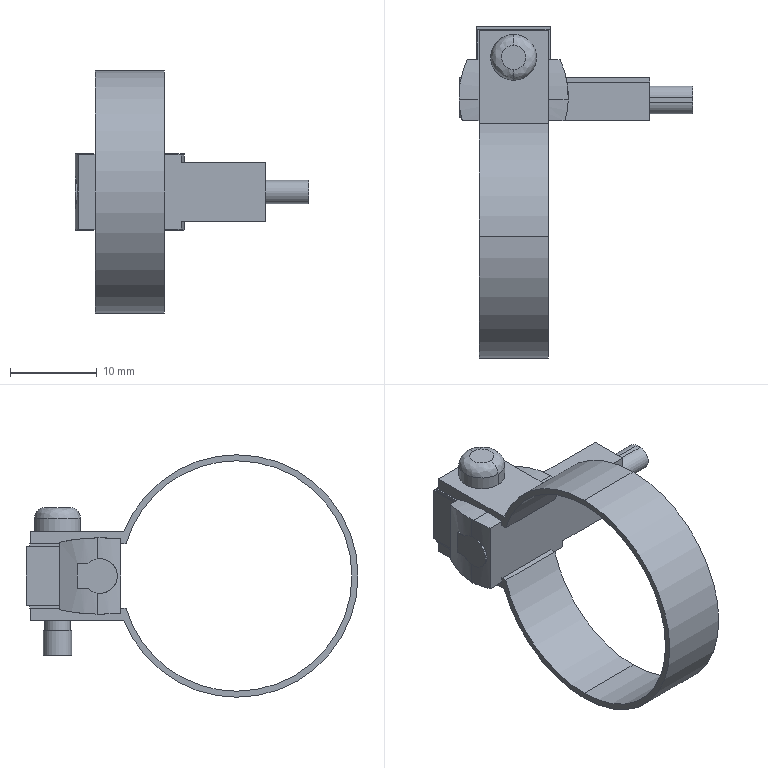Part | SolidWorks | features BaseBody 1 | 1 solid | 73 faces | box 27.005 x 38.33 x 28 mm | volume 2014 mm3 | plane 43 | cylinder 28 | spline 2 | commonest cylinder face diameters 44 x6 3 x4 4 x3 20.776 x3 26.6 x3 28 x3